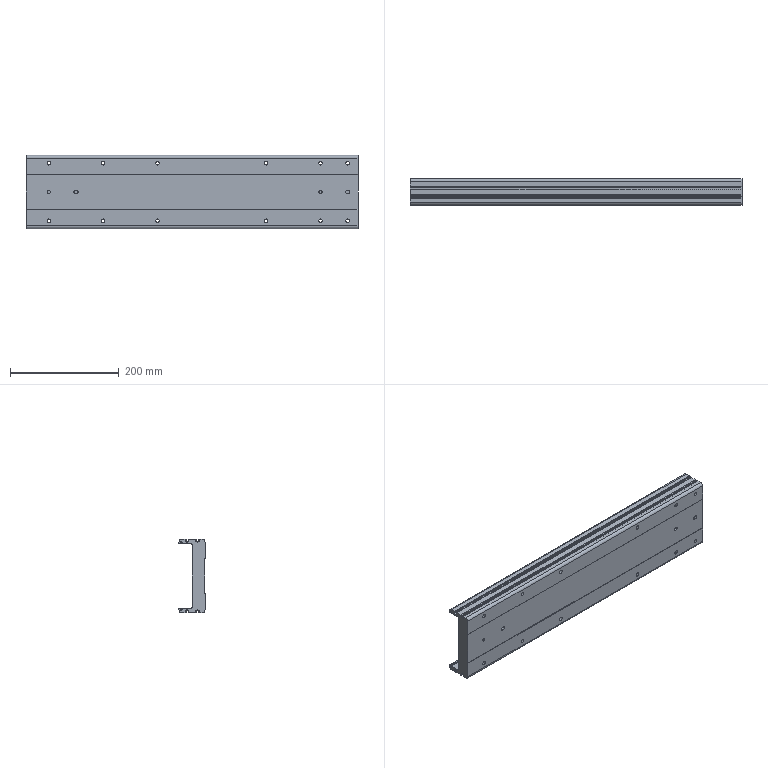Part | SolidWorks | features BaseBody 1 | 1 solid | 197 faces | box 611 x 48 x 135 mm | volume 2089073 mm3 | plane 96 | cylinder 77 | cone 24 | commonest cylinder face diameters 6.647 x24 11 x24 6 x8 4.2 x6 0.4 x4 10 x4